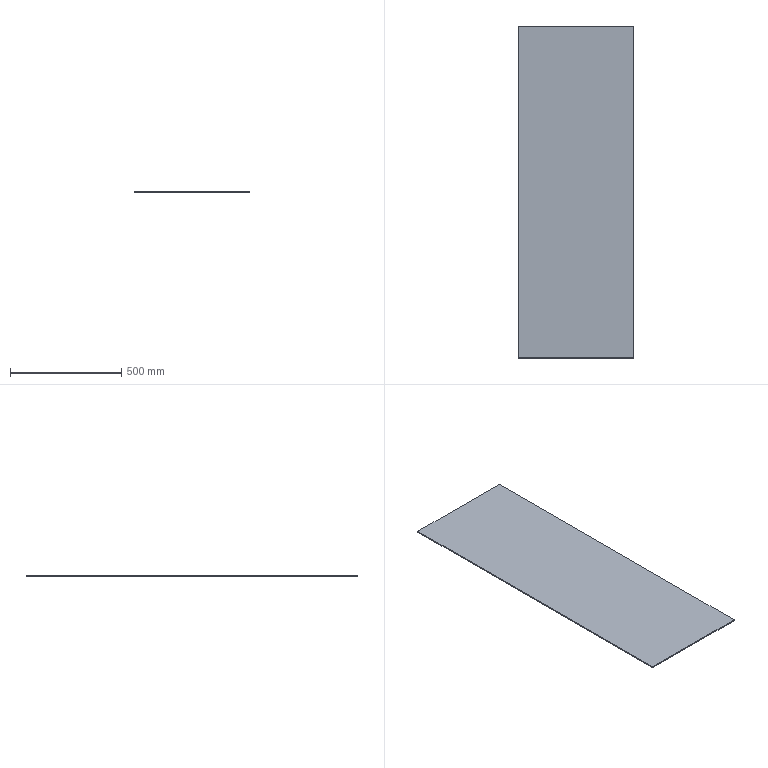Part | SolidWorks | features Extrusion 1, HoleWzd 1 | 1 solid | 6 faces | box 517 x 1491 x 5 mm | volume 3854235 mm3 | plane 6
STEP:
#1=CARTESIAN_POINT('',(258.5,-745.5,0.));
#2=VERTEX_POINT('',#1);
#3=CARTESIAN_POINT('',(258.5,745.5,0.));
#4=VERTEX_POINT('',#3);
#5=CARTESIAN_POINT('',(258.5,745.5,0.));
#6=DIRECTION('',(0.,1.,0.));
#7=VECTOR('',#6,1000.);
#8=LINE('',#5,#7);
#9=EDGE_CURVE('',#2,#4,#8,.T.);
#10=ORIENTED_EDGE('',*,*,#9,.T.);
#11=CARTESIAN_POINT('',(258.5,745.5,5.));
#12=VERTEX_POINT('',#11);
#13=CARTESIAN_POINT('',(258.5,745.5,5.));
#14=DIRECTION('',(0.,0.,-1.));
#15=VECTOR('',#14,1000.);
#16=LINE('',#13,#15);
#17=EDGE_CURVE('',#12,#4,#16,.T.);
#18=ORIENTED_EDGE('',*,*,#17,.F.);
#19=CARTESIAN_POINT('',(258.5,-745.5,5.));
#20=VERTEX_POINT('',#19);
#21=CARTESIAN_POINT('',(258.5,745.5,5.));
#22=DIRECTION('',(0.,1.,0.));
#23=VECTOR('',#22,1000.);
#24=LINE('',#21,#23);
#25=EDGE_CURVE('',#20,#12,#24,.T.);
#26=ORIENTED_EDGE('',*,*,#25,.F.);
#27=CARTESIAN_POINT('',(258.5,-745.5,5.));
#28=DIRECTION('',(0.,0.,-1.));
#29=VECTOR('',#28,1000.);
#30=LINE('',#27,#29);
#31=EDGE_CURVE('',#20,#2,#30,.T.);
#32=ORIENTED_EDGE('',*,*,#31,.T.);
#33=EDGE_LOOP('',(#10,#18,#26,#32));
#34=FACE_OUTER_BOUND('',#33,.T.);
#35=CARTESIAN_POINT('',(258.5,745.5,5.));
#36=DIRECTION('',(-1.,0.,0.));
#37=DIRECTION('',(0.,-1.,0.));
#38=AXIS2_PLACEMENT_3D('',#35,#36,#37);
#39=PLANE('',#38);
#40=ADVANCED_FACE('',(#34),#39,.F.);
#41=CARTESIAN_POINT('',(-258.5,745.5,0.));
#42=VERTEX_POINT('',#41);
#43=CARTESIAN_POINT('',(-258.5,745.5,0.));
#44=DIRECTION('',(-1.,0.,0.));
#45=VECTOR('',#44,1000.);
#46=LINE('',#43,#45);
#47=EDGE_CURVE('',#4,#42,#46,.T.);
#48=ORIENTED_EDGE('',*,*,#47,.T.);
#49=CARTESIAN_POINT('',(-258.5,745.5,5.));
#50=VERTEX_POINT('',#49);
#51=CARTESIAN_POINT('',(-258.5,745.5,5.));
#52=DIRECTION('',(0.,0.,-1.));
#53=VECTOR('',#52,1000.);
#54=LINE('',#51,#53);
#55=EDGE_CURVE('',#50,#42,#54,.T.);
#56=ORIENTED_EDGE('',*,*,#55,.F.);
#57=CARTESIAN_POINT('',(-258.5,745.5,5.));
#58=DIRECTION('',(-1.,0.,0.));
#59=VECTOR('',#58,1000.);
#60=LINE('',#57,#59);
#61=EDGE_CURVE('',#12,#50,#60,.T.);
#62=ORIENTED_EDGE('',*,*,#61,.F.);
#63=ORIENTED_EDGE('',*,*,#17,.T.);
#64=EDGE_LOOP('',(#48,#56,#62,#63));
#65=FACE_OUTER_BOUND('',#64,.T.);
#66=CARTESIAN_POINT('',(-258.5,745.5,5.));
#67=DIRECTION('',(0.,-1.,0.));
#68=DIRECTION('',(0.,0.,-1.));
#69=AXIS2_PLACEMENT_3D('',#66,#67,#68);
#70=PLANE('',#69);
#71=ADVANCED_FACE('',(#65),#70,.F.);
#72=CARTESIAN_POINT('',(-258.5,-745.5,0.));
#73=VERTEX_POINT('',#72);
#74=CARTESIAN_POINT('',(-258.5,745.5,0.));
#75=DIRECTION('',(0.,-1.,0.));
#76=VECTOR('',#75,1000.);
#77=LINE('',#74,#76);
#78=EDGE_CURVE('',#42,#73,#77,.T.);
#79=ORIENTED_EDGE('',*,*,#78,.T.);
#80=CARTESIAN_POINT('',(-258.5,-745.5,5.));
#81=VERTEX_POINT('',#80);
#82=CARTESIAN_POINT('',(-258.5,-745.5,5.));
#83=DIRECTION('',(0.,0.,-1.));
#84=VECTOR('',#83,1000.);
#85=LINE('',#82,#84);
#86=EDGE_CURVE('',#81,#73,#85,.T.);
#87=ORIENTED_EDGE('',*,*,#86,.F.);
#88=CARTESIAN_POINT('',(-258.5,745.5,5.));
#89=DIRECTION('',(0.,-1.,0.));
#90=VECTOR('',#89,1000.);
#91=LINE('',#88,#90);
#92=EDGE_CURVE('',#50,#81,#91,.T.);
#93=ORIENTED_EDGE('',*,*,#92,.F.);
#94=ORIENTED_EDGE('',*,*,#55,.T.);
#95=EDGE_LOOP('',(#79,#87,#93,#94));
#96=FACE_OUTER_BOUND('',#95,.T.);
#97=CARTESIAN_POINT('',(-258.5,745.5,5.));
#98=DIRECTION('',(1.,0.,0.));
#99=DIRECTION('',(0.,1.,0.));
#100=AXIS2_PLACEMENT_3D('',#97,#98,#99);
#101=PLANE('',#100);
#102=ADVANCED_FACE('',(#96),#101,.F.);
#103=CARTESIAN_POINT('',(-258.5,-745.5,0.));
#104=DIRECTION('',(1.,0.,0.));
#105=VECTOR('',#104,1000.);
#106=LINE('',#103,#105);
#107=EDGE_CURVE('',#73,#2,#106,.T.);
#108=ORIENTED_EDGE('',*,*,#107,.T.);
#109=ORIENTED_EDGE('',*,*,#31,.F.);
#110=CARTESIAN_POINT('',(-258.5,-745.5,5.));
#111=DIRECTION('',(1.,0.,0.));
#112=VECTOR('',#111,1000.);
#113=LINE('',#110,#112);
#114=EDGE_CURVE('',#81,#20,#113,.T.);
#115=ORIENTED_EDGE('',*,*,#114,.F.);
#116=ORIENTED_EDGE('',*,*,#86,.T.);
#117=EDGE_LOOP('',(#108,#109,#115,#116));
#118=FACE_OUTER_BOUND('',#117,.T.);
#119=CARTESIAN_POINT('',(-258.5,-745.5,5.));
#120=DIRECTION('',(0.,1.,0.));
#121=DIRECTION('',(0.,0.,1.));
#122=AXIS2_PLACEMENT_3D('',#119,#120,#121);
#123=PLANE('',#122);
#124=ADVANCED_FACE('',(#118),#123,.F.);
#125=ORIENTED_EDGE('',*,*,#25,.T.);
#126=ORIENTED_EDGE('',*,*,#61,.T.);
#127=ORIENTED_EDGE('',*,*,#92,.T.);
#128=ORIENTED_EDGE('',*,*,#114,.T.);
#129=EDGE_LOOP('',(#125,#126,#127,#128));
#130=FACE_OUTER_BOUND('',#129,.T.);
#131=CARTESIAN_POINT('',(0.,0.,5.));
#132=DIRECTION('',(0.,0.,1.));
#133=DIRECTION('',(1.,0.,0.));
#134=AXIS2_PLACEMENT_3D('',#131,#132,#133);
#135=PLANE('',#134);
#136=ADVANCED_FACE('',(#130),#135,.T.);
#137=ORIENTED_EDGE('',*,*,#9,.F.);
#138=ORIENTED_EDGE('',*,*,#107,.F.);
#139=ORIENTED_EDGE('',*,*,#78,.F.);
#140=ORIENTED_EDGE('',*,*,#47,.F.);
#141=EDGE_LOOP('',(#137,#138,#139,#140));
#142=FACE_OUTER_BOUND('',#141,.T.);
#143=CARTESIAN_POINT('',(0.,0.,0.));
#144=DIRECTION('',(0.,0.,1.));
#145=DIRECTION('',(1.,0.,0.));
#146=AXIS2_PLACEMENT_3D('',#143,#144,#145);
#147=PLANE('',#146);
#148=ADVANCED_FACE('',(#142),#147,.F.);
#149=CLOSED_SHELL('',(#40,#71,#102,#124,#136,#148));
#150=MANIFOLD_SOLID_BREP('',#149);
#151=CARTESIAN_POINT('',(0.,0.,0.));
#152=DIRECTION('',(0.,0.,1.));
#153=DIRECTION('',(1.,0.,0.));
#154=AXIS2_PLACEMENT_3D('',#151,#152,#153);
#155=(LENGTH_UNIT()NAMED_UNIT(*)SI_UNIT(.MILLI.,.METRE.));
#156=UNCERTAINTY_MEASURE_WITH_UNIT(LENGTH_MEASURE(0.00001),#155,'','');
#157=(NAMED_UNIT(*)PLANE_ANGLE_UNIT()SI_UNIT($,.RADIAN.));
#158=(NAMED_UNIT(*)SI_UNIT($,.STERADIAN.)SOLID_ANGLE_UNIT());
#159=(GEOMETRIC_REPRESENTATION_CONTEXT(3)GLOBAL_UNCERTAINTY_ASSIGNED_CONTEXT((#156))GLOBAL_UNIT_ASSIGNED_CONTEXT((#155,#157,#158))REPRESENTATION_CONTEXT('',''));
#160=ADVANCED_BREP_SHAPE_REPRESENTATION('',(#150,#154),#159);